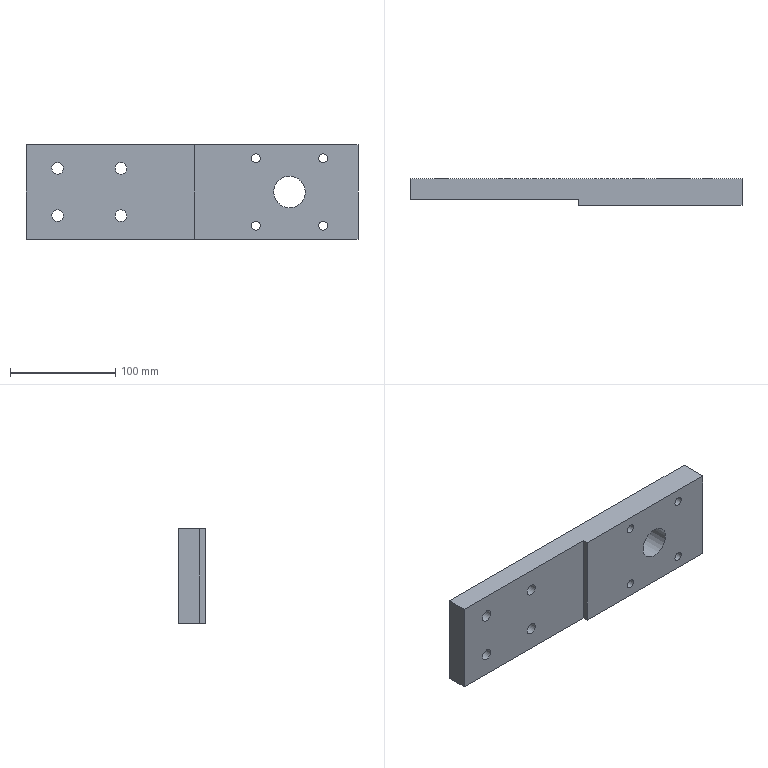Part | STEP file | SN10_002_001_PLACA | 1 solid | 17 faces | box 315 x 25 x 90 mm | volume 605966 mm3 | cylinder 9 | plane 8 | commonest cylinder face diameters 8.376 x4 11 x4 30 x1
STEP:
#1=CARTESIAN_POINT('',(0.,0.,0.));
#2=DIRECTION('',(0.,0.,1.));
#3=DIRECTION('',(1.,0.,0.));
#4=AXIS2_PLACEMENT_3D('',#1,#2,#3);
#5=CARTESIAN_POINT('',(5784.827,200.,-19.863));
#6=VERTEX_POINT('',#5);
#7=CARTESIAN_POINT('',(5780.,200.,-22.5));
#8=DIRECTION('',(0.,-1.,0.));
#9=DIRECTION('',(1.,0.,0.));
#10=AXIS2_PLACEMENT_3D('',#7,#8,#9);
#11=CIRCLE('',#10,5.5);
#12=CARTESIAN_POINT('',(5780.,199.9,-22.5));
#13=DIRECTION('',(0.,-1.,0.));
#14=DIRECTION('',(0.8776,0.,0.4794));
#15=AXIS2_PLACEMENT_3D('',#12,#13,#14);
#16=CYLINDRICAL_SURFACE('',#15,5.5);
#17=CARTESIAN_POINT('',(-0.5,-0.1));
#18=DIRECTION('',(1.,0.));
#19=VECTOR('',#18,1.);
#20=LINE('',#17,#19);
#21=(GEOMETRIC_REPRESENTATION_CONTEXT(2)PARAMETRIC_REPRESENTATION_CONTEXT()REPRESENTATION_CONTEXT('',''));
#22=DEFINITIONAL_REPRESENTATION('',(#20),#21);
#23=PCURVE('',#16,#22);
#24=CARTESIAN_POINT('',(6065.,200.,0.));
#25=DIRECTION('',(0.,1.,0.));
#26=DIRECTION('',(0.,0.,1.));
#27=AXIS2_PLACEMENT_3D('',#24,#25,#26);
#28=PLANE('',#27);
#29=CARTESIAN_POINT('',(-22.5,-279.5));
#30=CARTESIAN_POINT('',(-12.974,-279.5));
#31=CARTESIAN_POINT('',(-17.737,-287.75));
#32=CARTESIAN_POINT('',(-22.5,-296.));
#33=CARTESIAN_POINT('',(-27.263,-287.75));
#34=CARTESIAN_POINT('',(-32.026,-279.5));
#35=CARTESIAN_POINT('',(-22.5,-279.5));
#36=(BOUNDED_CURVE()B_SPLINE_CURVE(2,(#29,#30,#31,#32,#33,#34,#35),.UNSPECIFIED.,.T.,.F.)B_SPLINE_CURVE_WITH_KNOTS((1,2,2,2,2,1),(-2.094,0.,2.094,4.189,6.283,8.378),.UNSPECIFIED.)CURVE()GEOMETRIC_REPRESENTATION_ITEM()RATIONAL_B_SPLINE_CURVE((1.,0.5,1.,0.5,1.,0.5,1.))REPRESENTATION_ITEM(''));
#37=(GEOMETRIC_REPRESENTATION_CONTEXT(2)PARAMETRIC_REPRESENTATION_CONTEXT()REPRESENTATION_CONTEXT('',''));
#38=DEFINITIONAL_REPRESENTATION('',(#36),#37);
#39=PCURVE('',#28,#38);
#40=SURFACE_CURVE('',#11,(#23,#39),.PCURVE_S1.);
#41=EDGE_CURVE('',#6,#6,#40,.T.);
#42=ORIENTED_EDGE('',*,*,#41,.T.);
#43=CARTESIAN_POINT('',(5784.827,180.,-19.863));
#44=VERTEX_POINT('',#43);
#45=CARTESIAN_POINT('',(5784.827,200.,-19.863));
#46=CARTESIAN_POINT('',(5784.827,180.,-19.863));
#47=B_SPLINE_CURVE_WITH_KNOTS('',1,(#45,#46),.UNSPECIFIED.,.F.,.F.,(2,2),(-0.1,19.9),.PIECEWISE_BEZIER_KNOTS.);
#48=CARTESIAN_POINT('',(6.283,0.));
#49=DIRECTION('',(0.,1.));
#50=VECTOR('',#49,1.);
#51=LINE('',#48,#50);
#52=(GEOMETRIC_REPRESENTATION_CONTEXT(2)PARAMETRIC_REPRESENTATION_CONTEXT()REPRESENTATION_CONTEXT('',''));
#53=DEFINITIONAL_REPRESENTATION('',(#51),#52);
#54=PCURVE('',#16,#53);
#55=CARTESIAN_POINT('',(0.,0.));
#56=DIRECTION('',(0.,1.));
#57=VECTOR('',#56,1.);
#58=LINE('',#55,#57);
#59=(GEOMETRIC_REPRESENTATION_CONTEXT(2)PARAMETRIC_REPRESENTATION_CONTEXT()REPRESENTATION_CONTEXT('',''));
#60=DEFINITIONAL_REPRESENTATION('',(#58),#59);
#61=PCURVE('',#16,#60);
#62=SEAM_CURVE('',#47,(#54,#61),.PCURVE_S1.);
#63=EDGE_CURVE('',#6,#44,#62,.T.);
#64=ORIENTED_EDGE('',*,*,#63,.T.);
#65=CARTESIAN_POINT('',(5780.,180.,-22.5));
#66=DIRECTION('',(0.,-1.,0.));
#67=DIRECTION('',(1.,0.,0.));
#68=AXIS2_PLACEMENT_3D('',#65,#66,#67);
#69=CIRCLE('',#68,5.5);
#70=CARTESIAN_POINT('',(-0.5,19.9));
#71=DIRECTION('',(1.,0.));
#72=VECTOR('',#71,1.);
#73=LINE('',#70,#72);
#74=(GEOMETRIC_REPRESENTATION_CONTEXT(2)PARAMETRIC_REPRESENTATION_CONTEXT()REPRESENTATION_CONTEXT('',''));
#75=DEFINITIONAL_REPRESENTATION('',(#73),#74);
#76=PCURVE('',#16,#75);
#77=CARTESIAN_POINT('',(5750.,180.,0.));
#78=DIRECTION('',(0.,-1.,0.));
#79=DIRECTION('',(0.,0.,-1.));
#80=AXIS2_PLACEMENT_3D('',#77,#78,#79);
#81=PLANE('',#80);
#82=CARTESIAN_POINT('',(22.5,30.));
#83=DIRECTION('',(0.,1.));
#84=AXIS2_PLACEMENT_2D('',#82,#83);
#85=CIRCLE('',#84,5.5);
#86=(GEOMETRIC_REPRESENTATION_CONTEXT(2)PARAMETRIC_REPRESENTATION_CONTEXT()REPRESENTATION_CONTEXT('',''));
#87=DEFINITIONAL_REPRESENTATION('',(#85),#86);
#88=PCURVE('',#81,#87);
#89=SURFACE_CURVE('',#69,(#76,#88),.PCURVE_S1.);
#90=EDGE_CURVE('',#44,#44,#89,.T.);
#91=ORIENTED_EDGE('',*,*,#90,.F.);
#92=ORIENTED_EDGE('',*,*,#63,.F.);
#93=EDGE_LOOP('',(#42,#64,#91,#92));
#94=FACE_BOUND('',#93,.F.);
#95=ADVANCED_FACE('',(#94),#16,.F.);
#96=CARTESIAN_POINT('',(5750.,200.,-45.));
#97=VERTEX_POINT('',#96);
#98=CARTESIAN_POINT('',(5750.,180.,-45.));
#99=VERTEX_POINT('',#98);
#100=CARTESIAN_POINT('',(5750.,200.,-45.));
#101=DIRECTION('',(0.,-1.,0.));
#102=VECTOR('',#101,1.);
#103=LINE('',#100,#102);
#104=CARTESIAN_POINT('',(0.,0.,-45.));
#105=DIRECTION('',(0.,0.,1.));
#106=DIRECTION('',(1.,0.,0.));
#107=AXIS2_PLACEMENT_3D('',#104,#105,#106);
#108=PLANE('',#107);
#109=CARTESIAN_POINT('',(5750.,200.));
#110=DIRECTION('',(0.,-1.));
#111=VECTOR('',#110,1.);
#112=LINE('',#109,#111);
#113=(GEOMETRIC_REPRESENTATION_CONTEXT(2)PARAMETRIC_REPRESENTATION_CONTEXT()REPRESENTATION_CONTEXT('',''));
#114=DEFINITIONAL_REPRESENTATION('',(#112),#113);
#115=PCURVE('',#108,#114);
#116=CARTESIAN_POINT('',(5750.,200.,0.));
#117=DIRECTION('',(-1.,0.,0.));
#118=DIRECTION('',(0.,0.,1.));
#119=AXIS2_PLACEMENT_3D('',#116,#117,#118);
#120=PLANE('',#119);
#121=CARTESIAN_POINT('',(-45.,0.));
#122=DIRECTION('',(0.,-1.));
#123=VECTOR('',#122,1.);
#124=LINE('',#121,#123);
#125=(GEOMETRIC_REPRESENTATION_CONTEXT(2)PARAMETRIC_REPRESENTATION_CONTEXT()REPRESENTATION_CONTEXT('',''));
#126=DEFINITIONAL_REPRESENTATION('',(#124),#125);
#127=PCURVE('',#120,#126);
#128=SURFACE_CURVE('',#103,(#115,#127),.PCURVE_S1.);
#129=EDGE_CURVE('',#97,#99,#128,.T.);
#130=ORIENTED_EDGE('',*,*,#129,.F.);
#131=CARTESIAN_POINT('',(6065.,200.,-45.));
#132=VERTEX_POINT('',#131);
#133=CARTESIAN_POINT('',(6065.,200.,-45.));
#134=DIRECTION('',(-1.,0.,0.));
#135=VECTOR('',#134,1.);
#136=LINE('',#133,#135);
#137=CARTESIAN_POINT('',(6065.,200.));
#138=DIRECTION('',(-1.,0.));
#139=VECTOR('',#138,1.);
#140=LINE('',#137,#139);
#141=(GEOMETRIC_REPRESENTATION_CONTEXT(2)PARAMETRIC_REPRESENTATION_CONTEXT()REPRESENTATION_CONTEXT('',''));
#142=DEFINITIONAL_REPRESENTATION('',(#140),#141);
#143=PCURVE('',#108,#142);
#144=CARTESIAN_POINT('',(-45.,0.));
#145=DIRECTION('',(0.,-1.));
#146=VECTOR('',#145,1.);
#147=LINE('',#144,#146);
#148=(GEOMETRIC_REPRESENTATION_CONTEXT(2)PARAMETRIC_REPRESENTATION_CONTEXT()REPRESENTATION_CONTEXT('',''));
#149=DEFINITIONAL_REPRESENTATION('',(#147),#148);
#150=PCURVE('',#28,#149);
#151=SURFACE_CURVE('',#136,(#143,#150),.PCURVE_S1.);
#152=EDGE_CURVE('',#132,#97,#151,.T.);
#153=ORIENTED_EDGE('',*,*,#152,.F.);
#154=CARTESIAN_POINT('',(6065.,175.,-45.));
#155=VERTEX_POINT('',#154);
#156=CARTESIAN_POINT('',(6065.,175.,-45.));
#157=DIRECTION('',(0.,1.,0.));
#158=VECTOR('',#157,1.);
#159=LINE('',#156,#158);
#160=CARTESIAN_POINT('',(6065.,175.));
#161=DIRECTION('',(0.,1.));
#162=VECTOR('',#161,1.);
#163=LINE('',#160,#162);
#164=(GEOMETRIC_REPRESENTATION_CONTEXT(2)PARAMETRIC_REPRESENTATION_CONTEXT()REPRESENTATION_CONTEXT('',''));
#165=DEFINITIONAL_REPRESENTATION('',(#163),#164);
#166=PCURVE('',#108,#165);
#167=CARTESIAN_POINT('',(6065.,175.,0.));
#168=DIRECTION('',(1.,0.,0.));
#169=DIRECTION('',(0.,0.,-1.));
#170=AXIS2_PLACEMENT_3D('',#167,#168,#169);
#171=PLANE('',#170);
#172=CARTESIAN_POINT('',(45.,0.));
#173=DIRECTION('',(0.,1.));
#174=VECTOR('',#173,1.);
#175=LINE('',#172,#174);
#176=(GEOMETRIC_REPRESENTATION_CONTEXT(2)PARAMETRIC_REPRESENTATION_CONTEXT()REPRESENTATION_CONTEXT('',''));
#177=DEFINITIONAL_REPRESENTATION('',(#175),#176);
#178=PCURVE('',#171,#177);
#179=SURFACE_CURVE('',#159,(#166,#178),.PCURVE_S1.);
#180=EDGE_CURVE('',#155,#132,#179,.T.);
#181=ORIENTED_EDGE('',*,*,#180,.F.);
#182=CARTESIAN_POINT('',(5910.,175.,-45.));
#183=VERTEX_POINT('',#182);
#184=CARTESIAN_POINT('',(5910.,175.,-45.));
#185=DIRECTION('',(1.,0.,0.));
#186=VECTOR('',#185,1.);
#187=LINE('',#184,#186);
#188=CARTESIAN_POINT('',(5910.,175.));
#189=DIRECTION('',(1.,0.));
#190=VECTOR('',#189,1.);
#191=LINE('',#188,#190);
#192=(GEOMETRIC_REPRESENTATION_CONTEXT(2)PARAMETRIC_REPRESENTATION_CONTEXT()REPRESENTATION_CONTEXT('',''));
#193=DEFINITIONAL_REPRESENTATION('',(#191),#192);
#194=PCURVE('',#108,#193);
#195=CARTESIAN_POINT('',(5910.,175.,0.));
#196=DIRECTION('',(0.,-1.,0.));
#197=DIRECTION('',(0.,0.,-1.));
#198=AXIS2_PLACEMENT_3D('',#195,#196,#197);
#199=PLANE('',#198);
#200=CARTESIAN_POINT('',(45.,0.));
#201=DIRECTION('',(0.,1.));
#202=VECTOR('',#201,1.);
#203=LINE('',#200,#202);
#204=(GEOMETRIC_REPRESENTATION_CONTEXT(2)PARAMETRIC_REPRESENTATION_CONTEXT()REPRESENTATION_CONTEXT('',''));
#205=DEFINITIONAL_REPRESENTATION('',(#203),#204);
#206=PCURVE('',#199,#205);
#207=SURFACE_CURVE('',#187,(#194,#206),.PCURVE_S1.);
#208=EDGE_CURVE('',#183,#155,#207,.T.);
#209=ORIENTED_EDGE('',*,*,#208,.F.);
#210=CARTESIAN_POINT('',(5910.,180.,-45.));
#211=VERTEX_POINT('',#210);
#212=CARTESIAN_POINT('',(5910.,180.,-45.));
#213=DIRECTION('',(0.,-1.,0.));
#214=VECTOR('',#213,1.);
#215=LINE('',#212,#214);
#216=CARTESIAN_POINT('',(5910.,180.));
#217=DIRECTION('',(0.,-1.));
#218=VECTOR('',#217,1.);
#219=LINE('',#216,#218);
#220=(GEOMETRIC_REPRESENTATION_CONTEXT(2)PARAMETRIC_REPRESENTATION_CONTEXT()REPRESENTATION_CONTEXT('',''));
#221=DEFINITIONAL_REPRESENTATION('',(#219),#220);
#222=PCURVE('',#108,#221);
#223=CARTESIAN_POINT('',(5910.,180.,0.));
#224=DIRECTION('',(-1.,0.,0.));
#225=DIRECTION('',(0.,0.,1.));
#226=AXIS2_PLACEMENT_3D('',#223,#224,#225);
#227=PLANE('',#226);
#228=CARTESIAN_POINT('',(-45.,0.));
#229=DIRECTION('',(0.,-1.));
#230=VECTOR('',#229,1.);
#231=LINE('',#228,#230);
#232=(GEOMETRIC_REPRESENTATION_CONTEXT(2)PARAMETRIC_REPRESENTATION_CONTEXT()REPRESENTATION_CONTEXT('',''));
#233=DEFINITIONAL_REPRESENTATION('',(#231),#232);
#234=PCURVE('',#227,#233);
#235=SURFACE_CURVE('',#215,(#222,#234),.PCURVE_S1.);
#236=EDGE_CURVE('',#211,#183,#235,.T.);
#237=ORIENTED_EDGE('',*,*,#236,.F.);
#238=CARTESIAN_POINT('',(5750.,180.,-45.));
#239=DIRECTION('',(1.,0.,0.));
#240=VECTOR('',#239,1.);
#241=LINE('',#238,#240);
#242=CARTESIAN_POINT('',(5750.,180.));
#243=DIRECTION('',(1.,0.));
#244=VECTOR('',#243,1.);
#245=LINE('',#242,#244);
#246=(GEOMETRIC_REPRESENTATION_CONTEXT(2)PARAMETRIC_REPRESENTATION_CONTEXT()REPRESENTATION_CONTEXT('',''));
#247=DEFINITIONAL_REPRESENTATION('',(#245),#246);
#248=PCURVE('',#108,#247);
#249=CARTESIAN_POINT('',(45.,0.));
#250=DIRECTION('',(0.,1.));
#251=VECTOR('',#250,1.);
#252=LINE('',#249,#251);
#253=(GEOMETRIC_REPRESENTATION_CONTEXT(2)PARAMETRIC_REPRESENTATION_CONTEXT()REPRESENTATION_CONTEXT('',''));
#254=DEFINITIONAL_REPRESENTATION('',(#252),#253);
#255=PCURVE('',#81,#254);
#256=SURFACE_CURVE('',#241,(#248,#255),.PCURVE_S1.);
#257=EDGE_CURVE('',#99,#211,#256,.T.);
#258=ORIENTED_EDGE('',*,*,#257,.F.);
#259=EDGE_LOOP('',(#130,#153,#181,#209,#237,#258));
#260=FACE_BOUND('',#259,.T.);
#261=ADVANCED_FACE('',(#260),#108,.F.);
#262=CARTESIAN_POINT('',(5750.,200.,45.));
#263=VERTEX_POINT('',#262);
#264=CARTESIAN_POINT('',(5750.,200.,-45.));
#265=DIRECTION('',(0.,0.,1.));
#266=VECTOR('',#265,1.);
#267=LINE('',#264,#266);
#268=CARTESIAN_POINT('',(-45.,0.));
#269=DIRECTION('',(1.,0.));
#270=VECTOR('',#269,1.);
#271=LINE('',#268,#270);
#272=(GEOMETRIC_REPRESENTATION_CONTEXT(2)PARAMETRIC_REPRESENTATION_CONTEXT()REPRESENTATION_CONTEXT('',''));
#273=DEFINITIONAL_REPRESENTATION('',(#271),#272);
#274=PCURVE('',#120,#273);
#275=CARTESIAN_POINT('',(-45.,-315.));
#276=DIRECTION('',(1.,0.));
#277=VECTOR('',#276,1.);
#278=LINE('',#275,#277);
#279=(GEOMETRIC_REPRESENTATION_CONTEXT(2)PARAMETRIC_REPRESENTATION_CONTEXT()REPRESENTATION_CONTEXT('',''));
#280=DEFINITIONAL_REPRESENTATION('',(#278),#279);
#281=PCURVE('',#28,#280);
#282=SURFACE_CURVE('',#267,(#274,#281),.PCURVE_S1.);
#283=EDGE_CURVE('',#97,#263,#282,.T.);
#284=ORIENTED_EDGE('',*,*,#283,.F.);
#285=ORIENTED_EDGE('',*,*,#129,.T.);
#286=CARTESIAN_POINT('',(5750.,180.,45.));
#287=VERTEX_POINT('',#286);
#288=CARTESIAN_POINT('',(5750.,180.,-45.));
#289=DIRECTION('',(0.,0.,1.));
#290=VECTOR('',#289,1.);
#291=LINE('',#288,#290);
#292=CARTESIAN_POINT('',(-45.,-20.));
#293=DIRECTION('',(1.,0.));
#294=VECTOR('',#293,1.);
#295=LINE('',#292,#294);
#296=(GEOMETRIC_REPRESENTATION_CONTEXT(2)PARAMETRIC_REPRESENTATION_CONTEXT()REPRESENTATION_CONTEXT('',''));
#297=DEFINITIONAL_REPRESENTATION('',(#295),#296);
#298=PCURVE('',#120,#297);
#299=CARTESIAN_POINT('',(45.,0.));
#300=DIRECTION('',(-1.,0.));
#301=VECTOR('',#300,1.);
#302=LINE('',#299,#301);
#303=(GEOMETRIC_REPRESENTATION_CONTEXT(2)PARAMETRIC_REPRESENTATION_CONTEXT()REPRESENTATION_CONTEXT('',''));
#304=DEFINITIONAL_REPRESENTATION('',(#302),#303);
#305=PCURVE('',#81,#304);
#306=SURFACE_CURVE('',#291,(#298,#305),.PCURVE_S1.);
#307=EDGE_CURVE('',#99,#287,#306,.T.);
#308=ORIENTED_EDGE('',*,*,#307,.T.);
#309=CARTESIAN_POINT('',(5750.,200.,45.));
#310=DIRECTION('',(0.,-1.,0.));
#311=VECTOR('',#310,1.);
#312=LINE('',#309,#311);
#313=CARTESIAN_POINT('',(45.,0.));
#314=DIRECTION('',(0.,-1.));
#315=VECTOR('',#314,1.);
#316=LINE('',#313,#315);
#317=(GEOMETRIC_REPRESENTATION_CONTEXT(2)PARAMETRIC_REPRESENTATION_CONTEXT()REPRESENTATION_CONTEXT('',''));
#318=DEFINITIONAL_REPRESENTATION('',(#316),#317);
#319=PCURVE('',#120,#318);
#320=CARTESIAN_POINT('',(0.,0.,45.));
#321=DIRECTION('',(0.,0.,1.));
#322=DIRECTION('',(1.,0.,0.));
#323=AXIS2_PLACEMENT_3D('',#320,#321,#322);
#324=PLANE('',#323);
#325=CARTESIAN_POINT('',(5750.,200.));
#326=DIRECTION('',(0.,-1.));
#327=VECTOR('',#326,1.);
#328=LINE('',#325,#327);
#329=(GEOMETRIC_REPRESENTATION_CONTEXT(2)PARAMETRIC_REPRESENTATION_CONTEXT()REPRESENTATION_CONTEXT('',''));
#330=DEFINITIONAL_REPRESENTATION('',(#328),#329);
#331=PCURVE('',#324,#330);
#332=SURFACE_CURVE('',#312,(#319,#331),.PCURVE_S1.);
#333=EDGE_CURVE('',#263,#287,#332,.T.);
#334=ORIENTED_EDGE('',*,*,#333,.F.);
#335=EDGE_LOOP('',(#284,#285,#308,#334));
#336=FACE_BOUND('',#335,.T.);
#337=ADVANCED_FACE('',(#336),#120,.T.);
#338=CARTESIAN_POINT('',(5910.,180.,45.));
#339=VERTEX_POINT('',#338);
#340=CARTESIAN_POINT('',(5910.,180.,-45.));
#341=DIRECTION('',(0.,0.,1.));
#342=VECTOR('',#341,1.);
#343=LINE('',#340,#342);
#344=CARTESIAN_POINT('',(-45.,0.));
#345=DIRECTION('',(1.,0.));
#346=VECTOR('',#345,1.);
#347=LINE('',#344,#346);
#348=(GEOMETRIC_REPRESENTATION_CONTEXT(2)PARAMETRIC_REPRESENTATION_CONTEXT()REPRESENTATION_CONTEXT('',''));
#349=DEFINITIONAL_REPRESENTATION('',(#347),#348);
#350=PCURVE('',#227,#349);
#351=CARTESIAN_POINT('',(45.,160.));
#352=DIRECTION('',(-1.,0.));
#353=VECTOR('',#352,1.);
#354=LINE('',#351,#353);
#355=(GEOMETRIC_REPRESENTATION_CONTEXT(2)PARAMETRIC_REPRESENTATION_CONTEXT()REPRESENTATION_CONTEXT('',''));
#356=DEFINITIONAL_REPRESENTATION('',(#354),#355);
#357=PCURVE('',#81,#356);
#358=SURFACE_CURVE('',#343,(#350,#357),.PCURVE_S1.);
#359=EDGE_CURVE('',#211,#339,#358,.T.);
#360=ORIENTED_EDGE('',*,*,#359,.F.);
#361=ORIENTED_EDGE('',*,*,#236,.T.);
#362=CARTESIAN_POINT('',(5910.,175.,45.));
#363=VERTEX_POINT('',#362);
#364=CARTESIAN_POINT('',(5910.,175.,-45.));
#365=DIRECTION('',(0.,0.,1.));
#366=VECTOR('',#365,1.);
#367=LINE('',#364,#366);
#368=CARTESIAN_POINT('',(-45.,-5.));
#369=DIRECTION('',(1.,0.));
#370=VECTOR('',#369,1.);
#371=LINE('',#368,#370);
#372=(GEOMETRIC_REPRESENTATION_CONTEXT(2)PARAMETRIC_REPRESENTATION_CONTEXT()REPRESENTATION_CONTEXT('',''));
#373=DEFINITIONAL_REPRESENTATION('',(#371),#372);
#374=PCURVE('',#227,#373);
#375=CARTESIAN_POINT('',(45.,0.));
#376=DIRECTION('',(-1.,0.));
#377=VECTOR('',#376,1.);
#378=LINE('',#375,#377);
#379=(GEOMETRIC_REPRESENTATION_CONTEXT(2)PARAMETRIC_REPRESENTATION_CONTEXT()REPRESENTATION_CONTEXT('',''));
#380=DEFINITIONAL_REPRESENTATION('',(#378),#379);
#381=PCURVE('',#199,#380);
#382=SURFACE_CURVE('',#367,(#374,#381),.PCURVE_S1.);
#383=EDGE_CURVE('',#183,#363,#382,.T.);
#384=ORIENTED_EDGE('',*,*,#383,.T.);
#385=CARTESIAN_POINT('',(5910.,180.,45.));
#386=DIRECTION('',(0.,-1.,0.));
#387=VECTOR('',#386,1.);
#388=LINE('',#385,#387);
#389=CARTESIAN_POINT('',(45.,0.));
#390=DIRECTION('',(0.,-1.));
#391=VECTOR('',#390,1.);
#392=LINE('',#389,#391);
#393=(GEOMETRIC_REPRESENTATION_CONTEXT(2)PARAMETRIC_REPRESENTATION_CONTEXT()REPRESENTATION_CONTEXT('',''));
#394=DEFINITIONAL_REPRESENTATION('',(#392),#393);
#395=PCURVE('',#227,#394);
#396=CARTESIAN_POINT('',(5910.,180.));
#397=DIRECTION('',(0.,-1.));
#398=VECTOR('',#397,1.);
#399=LINE('',#396,#398);
#400=(GEOMETRIC_REPRESENTATION_CONTEXT(2)PARAMETRIC_REPRESENTATION_CONTEXT()REPRESENTATION_CONTEXT('',''));
#401=DEFINITIONAL_REPRESENTATION('',(#399),#400);
#402=PCURVE('',#324,#401);
#403=SURFACE_CURVE('',#388,(#395,#402),.PCURVE_S1.);
#404=EDGE_CURVE('',#339,#363,#403,.T.);
#405=ORIENTED_EDGE('',*,*,#404,.F.);
#406=EDGE_LOOP('',(#360,#361,#384,#405));
#407=FACE_BOUND('',#406,.T.);
#408=ADVANCED_FACE('',(#407),#227,.T.);
#409=ORIENTED_EDGE('',*,*,#383,.F.);
#410=ORIENTED_EDGE('',*,*,#208,.T.);
#411=CARTESIAN_POINT('',(6065.,175.,45.));
#412=VERTEX_POINT('',#411);
#413=CARTESIAN_POINT('',(6065.,175.,-45.));
#414=DIRECTION('',(0.,0.,1.));
#415=VECTOR('',#414,1.);
#416=LINE('',#413,#415);
#417=CARTESIAN_POINT('',(45.,155.));
#418=DIRECTION('',(-1.,0.));
#419=VECTOR('',#418,1.);
#420=LINE('',#417,#419);
#421=(GEOMETRIC_REPRESENTATION_CONTEXT(2)PARAMETRIC_REPRESENTATION_CONTEXT()REPRESENTATION_CONTEXT('',''));
#422=DEFINITIONAL_REPRESENTATION('',(#420),#421);
#423=PCURVE('',#199,#422);
#424=CARTESIAN_POINT('',(45.,0.));
#425=DIRECTION('',(-1.,0.));
#426=VECTOR('',#425,1.);
#427=LINE('',#424,#426);
#428=(GEOMETRIC_REPRESENTATION_CONTEXT(2)PARAMETRIC_REPRESENTATION_CONTEXT()REPRESENTATION_CONTEXT('',''));
#429=DEFINITIONAL_REPRESENTATION('',(#427),#428);
#430=PCURVE('',#171,#429);
#431=SURFACE_CURVE('',#416,(#423,#430),.PCURVE_S1.);
#432=EDGE_CURVE('',#155,#412,#431,.T.);
#433=ORIENTED_EDGE('',*,*,#432,.T.);
#434=CARTESIAN_POINT('',(5910.,175.,45.));
#435=DIRECTION('',(1.,0.,0.));
#436=VECTOR('',#435,1.);
#437=LINE('',#434,#436);
#438=CARTESIAN_POINT('',(-45.,0.));
#439=DIRECTION('',(0.,1.));
#440=VECTOR('',#439,1.);
#441=LINE('',#438,#440);
#442=(GEOMETRIC_REPRESENTATION_CONTEXT(2)PARAMETRIC_REPRESENTATION_CONTEXT()REPRESENTATION_CONTEXT('',''));
#443=DEFINITIONAL_REPRESENTATION('',(#441),#442);
#444=PCURVE('',#199,#443);
#445=CARTESIAN_POINT('',(5910.,175.));
#446=DIRECTION('',(1.,0.));
#447=VECTOR('',#446,1.);
#448=LINE('',#445,#447);
#449=(GEOMETRIC_REPRESENTATION_CONTEXT(2)PARAMETRIC_REPRESENTATION_CONTEXT()REPRESENTATION_CONTEXT('',''));
#450=DEFINITIONAL_REPRESENTATION('',(#448),#449);
#451=PCURVE('',#324,#450);
#452=SURFACE_CURVE('',#437,(#444,#451),.PCURVE_S1.);
#453=EDGE_CURVE('',#363,#412,#452,.T.);
#454=ORIENTED_EDGE('',*,*,#453,.F.);
#455=EDGE_LOOP('',(#409,#410,#433,#454));
#456=FACE_BOUND('',#455,.T.);
#457=CARTESIAN_POINT('',(6035.675,175.,34.008));
#458=VERTEX_POINT('',#457);
#459=CARTESIAN_POINT('',(6032.,175.,32.));
#460=DIRECTION('',(0.,-1.,0.));
#461=DIRECTION('',(1.,0.,0.));
#462=AXIS2_PLACEMENT_3D('',#459,#460,#461);
#463=CIRCLE('',#462,4.188);
#464=CARTESIAN_POINT('',(-32.,122.));
#465=DIRECTION('',(0.,1.));
#466=AXIS2_PLACEMENT_2D('',#464,#465);
#467=CIRCLE('',#466,4.188);
#468=(GEOMETRIC_REPRESENTATION_CONTEXT(2)PARAMETRIC_REPRESENTATION_CONTEXT()REPRESENTATION_CONTEXT('',''));
#469=DEFINITIONAL_REPRESENTATION('',(#467),#468);
#470=PCURVE('',#199,#469);
#471=CARTESIAN_POINT('',(6032.,199.9,32.));
#472=DIRECTION('',(0.,-1.,0.));
#473=DIRECTION('',(0.8776,0.,0.4794));
#474=AXIS2_PLACEMENT_3D('',#471,#472,#473);
#475=CYLINDRICAL_SURFACE('',#474,4.188);
#476=CARTESIAN_POINT('',(-0.5,24.9));
#477=DIRECTION('',(1.,0.));
#478=VECTOR('',#477,1.);
#479=LINE('',#476,#478);
#480=(GEOMETRIC_REPRESENTATION_CONTEXT(2)PARAMETRIC_REPRESENTATION_CONTEXT()REPRESENTATION_CONTEXT('',''));
#481=DEFINITIONAL_REPRESENTATION('',(#479),#480);
#482=PCURVE('',#475,#481);
#483=SURFACE_CURVE('',#463,(#470,#482),.PCURVE_S1.);
#484=EDGE_CURVE('',#458,#458,#483,.T.);
#485=ORIENTED_EDGE('',*,*,#484,.F.);
#486=EDGE_LOOP('',(#485));
#487=FACE_BOUND('',#486,.T.);
#488=CARTESIAN_POINT('',(5971.675,175.,34.008));
#489=VERTEX_POINT('',#488);
#490=CARTESIAN_POINT('',(5968.,175.,32.));
#491=DIRECTION('',(0.,-1.,0.));
#492=DIRECTION('',(1.,0.,0.));
#493=AXIS2_PLACEMENT_3D('',#490,#491,#492);
#494=CIRCLE('',#493,4.188);
#495=CARTESIAN_POINT('',(-32.,58.));
#496=DIRECTION('',(0.,1.));
#497=AXIS2_PLACEMENT_2D('',#495,#496);
#498=CIRCLE('',#497,4.188);
#499=(GEOMETRIC_REPRESENTATION_CONTEXT(2)PARAMETRIC_REPRESENTATION_CONTEXT()REPRESENTATION_CONTEXT('',''));
#500=DEFINITIONAL_REPRESENTATION('',(#498),#499);
#501=PCURVE('',#199,#500);
#502=CARTESIAN_POINT('',(5968.,199.9,32.));
#503=DIRECTION('',(0.,-1.,0.));
#504=DIRECTION('',(0.8776,0.,0.4794));
#505=AXIS2_PLACEMENT_3D('',#502,#503,#504);
#506=CYLINDRICAL_SURFACE('',#505,4.188);
#507=CARTESIAN_POINT('',(-0.5,24.9));
#508=DIRECTION('',(1.,0.));
#509=VECTOR('',#508,1.);
#510=LINE('',#507,#509);
#511=(GEOMETRIC_REPRESENTATION_CONTEXT(2)PARAMETRIC_REPRESENTATION_CONTEXT()REPRESENTATION_CONTEXT('',''));
#512=DEFINITIONAL_REPRESENTATION('',(#510),#511);
#513=PCURVE('',#506,#512);
#514=SURFACE_CURVE('',#494,(#501,#513),.PCURVE_S1.);
#515=EDGE_CURVE('',#489,#489,#514,.T.);
#516=ORIENTED_EDGE('',*,*,#515,.F.);
#517=EDGE_LOOP('',(#516));
#518=FACE_BOUND('',#517,.T.);
#519=CARTESIAN_POINT('',(5971.675,175.,-29.992));
#520=VERTEX_POINT('',#519);
#521=CARTESIAN_POINT('',(5968.,175.,-32.));
#522=DIRECTION('',(0.,-1.,0.));
#523=DIRECTION('',(1.,0.,0.));
#524=AXIS2_PLACEMENT_3D('',#521,#522,#523);
#525=CIRCLE('',#524,4.188);
#526=CARTESIAN_POINT('',(32.,58.));
#527=DIRECTION('',(0.,1.));
#528=AXIS2_PLACEMENT_2D('',#526,#527);
#529=CIRCLE('',#528,4.188);
#530=(GEOMETRIC_REPRESENTATION_CONTEXT(2)PARAMETRIC_REPRESENTATION_CONTEXT()REPRESENTATION_CONTEXT('',''));
#531=DEFINITIONAL_REPRESENTATION('',(#529),#530);
#532=PCURVE('',#199,#531);
#533=CARTESIAN_POINT('',(5968.,199.9,-32.));
#534=DIRECTION('',(0.,-1.,0.));
#535=DIRECTION('',(0.8776,0.,0.4794));
#536=AXIS2_PLACEMENT_3D('',#533,#534,#535);
#537=CYLINDRICAL_SURFACE('',#536,4.188);
#538=CARTESIAN_POINT('',(-0.5,24.9));
#539=DIRECTION('',(1.,0.));
#540=VECTOR('',#539,1.);
#541=LINE('',#538,#540);
#542=(GEOMETRIC_REPRESENTATION_CONTEXT(2)PARAMETRIC_REPRESENTATION_CONTEXT()REPRESENTATION_CONTEXT('',''));
#543=DEFINITIONAL_REPRESENTATION('',(#541),#542);
#544=PCURVE('',#537,#543);
#545=SURFACE_CURVE('',#525,(#532,#544),.PCURVE_S1.);
#546=EDGE_CURVE('',#520,#520,#545,.T.);
#547=ORIENTED_EDGE('',*,*,#546,.F.);
#548=EDGE_LOOP('',(#547));
#549=FACE_BOUND('',#548,.T.);
#550=CARTESIAN_POINT('',(6035.675,175.,-29.992));
#551=VERTEX_POINT('',#550);
#552=CARTESIAN_POINT('',(6032.,175.,-32.));
#553=DIRECTION('',(0.,-1.,0.));
#554=DIRECTION('',(1.,0.,0.));
#555=AXIS2_PLACEMENT_3D('',#552,#553,#554);
#556=CIRCLE('',#555,4.188);
#557=CARTESIAN_POINT('',(32.,122.));
#558=DIRECTION('',(0.,1.));
#559=AXIS2_PLACEMENT_2D('',#557,#558);
#560=CIRCLE('',#559,4.188);
#561=(GEOMETRIC_REPRESENTATION_CONTEXT(2)PARAMETRIC_REPRESENTATION_CONTEXT()REPRESENTATION_CONTEXT('',''));
#562=DEFINITIONAL_REPRESENTATION('',(#560),#561);
#563=PCURVE('',#199,#562);
#564=CARTESIAN_POINT('',(6032.,199.9,-32.));
#565=DIRECTION('',(0.,-1.,0.));
#566=DIRECTION('',(0.8776,0.,0.4794));
#567=AXIS2_PLACEMENT_3D('',#564,#565,#566);
#568=CYLINDRICAL_SURFACE('',#567,4.188);
#569=CARTESIAN_POINT('',(-0.5,24.9));
#570=DIRECTION('',(1.,0.));
#571=VECTOR('',#570,1.);
#572=LINE('',#569,#571);
#573=(GEOMETRIC_REPRESENTATION_CONTEXT(2)PARAMETRIC_REPRESENTATION_CONTEXT()REPRESENTATION_CONTEXT('',''));
#574=DEFINITIONAL_REPRESENTATION('',(#572),#573);
#575=PCURVE('',#568,#574);
#576=SURFACE_CURVE('',#556,(#563,#575),.PCURVE_S1.);
#577=EDGE_CURVE('',#551,#551,#576,.T.);
#578=ORIENTED_EDGE('',*,*,#577,.F.);
#579=EDGE_LOOP('',(#578));
#580=FACE_BOUND('',#579,.T.);
#581=CARTESIAN_POINT('',(6013.164,175.,7.191));
#582=VERTEX_POINT('',#581);
#583=CARTESIAN_POINT('',(6000.,175.,0.));
#584=DIRECTION('',(0.,-1.,0.));
#585=DIRECTION('',(1.,0.,0.));
#586=AXIS2_PLACEMENT_3D('',#583,#584,#585);
#587=CIRCLE('',#586,15.);
#588=CARTESIAN_POINT('',(0.,90.));
#589=DIRECTION('',(0.,1.));
#590=AXIS2_PLACEMENT_2D('',#588,#589);
#591=CIRCLE('',#590,15.);
#592=(GEOMETRIC_REPRESENTATION_CONTEXT(2)PARAMETRIC_REPRESENTATION_CONTEXT()REPRESENTATION_CONTEXT('',''));
#593=DEFINITIONAL_REPRESENTATION('',(#591),#592);
#594=PCURVE('',#199,#593);
#595=CARTESIAN_POINT('',(6000.,199.9,0.));
#596=DIRECTION('',(0.,-1.,0.));
#597=DIRECTION('',(0.8776,0.,0.4794));
#598=AXIS2_PLACEMENT_3D('',#595,#596,#597);
#599=CYLINDRICAL_SURFACE('',#598,15.);
#600=CARTESIAN_POINT('',(-0.5,24.9));
#601=DIRECTION('',(1.,0.));
#602=VECTOR('',#601,1.);
#603=LINE('',#600,#602);
#604=(GEOMETRIC_REPRESENTATION_CONTEXT(2)PARAMETRIC_REPRESENTATION_CONTEXT()REPRESENTATION_CONTEXT('',''));
#605=DEFINITIONAL_REPRESENTATION('',(#603),#604);
#606=PCURVE('',#599,#605);
#607=SURFACE_CURVE('',#587,(#594,#606),.PCURVE_S1.);
#608=EDGE_CURVE('',#582,#582,#607,.T.);
#609=ORIENTED_EDGE('',*,*,#608,.F.);
#610=EDGE_LOOP('',(#609));
#611=FACE_BOUND('',#610,.T.);
#612=ADVANCED_FACE('',(#456,#487,#518,#549,#580,#611),#199,.T.);
#613=CARTESIAN_POINT('',(6013.164,200.,7.191));
#614=VERTEX_POINT('',#613);
#615=CARTESIAN_POINT('',(6000.,200.,0.));
#616=DIRECTION('',(0.,-1.,0.));
#617=DIRECTION('',(1.,0.,0.));
#618=AXIS2_PLACEMENT_3D('',#615,#616,#617);
#619=CIRCLE('',#618,15.);
#620=CARTESIAN_POINT('',(-0.5,-0.1));
#621=DIRECTION('',(1.,0.));
#622=VECTOR('',#621,1.);
#623=LINE('',#620,#622);
#624=(GEOMETRIC_REPRESENTATION_CONTEXT(2)PARAMETRIC_REPRESENTATION_CONTEXT()REPRESENTATION_CONTEXT('',''));
#625=DEFINITIONAL_REPRESENTATION('',(#623),#624);
#626=PCURVE('',#599,#625);
#627=CARTESIAN_POINT('',(0.,-50.));
#628=CARTESIAN_POINT('',(25.981,-50.));
#629=CARTESIAN_POINT('',(12.99,-72.5));
#630=CARTESIAN_POINT('',(0.,-95.));
#631=CARTESIAN_POINT('',(-12.99,-72.5));
#632=CARTESIAN_POINT('',(-25.981,-50.));
#633=CARTESIAN_POINT('',(0.,-50.));
#634=(BOUNDED_CURVE()B_SPLINE_CURVE(2,(#627,#628,#629,#630,#631,#632,#633),.UNSPECIFIED.,.T.,.F.)B_SPLINE_CURVE_WITH_KNOTS((1,2,2,2,2,1),(-2.094,0.,2.094,4.189,6.283,8.378),.UNSPECIFIED.)CURVE()GEOMETRIC_REPRESENTATION_ITEM()RATIONAL_B_SPLINE_CURVE((1.,0.5,1.,0.5,1.,0.5,1.))REPRESENTATION_ITEM(''));
#635=(GEOMETRIC_REPRESENTATION_CONTEXT(2)PARAMETRIC_REPRESENTATION_CONTEXT()REPRESENTATION_CONTEXT('',''));
#636=DEFINITIONAL_REPRESENTATION('',(#634),#635);
#637=PCURVE('',#28,#636);
#638=SURFACE_CURVE('',#619,(#626,#637),.PCURVE_S1.);
#639=EDGE_CURVE('',#614,#614,#638,.T.);
#640=ORIENTED_EDGE('',*,*,#639,.T.);
#641=CARTESIAN_POINT('',(6013.164,200.,7.191));
#642=CARTESIAN_POINT('',(6013.164,175.,7.191));
#643=B_SPLINE_CURVE_WITH_KNOTS('',1,(#641,#642),.UNSPECIFIED.,.F.,.F.,(2,2),(-0.1,24.9),.PIECEWISE_BEZIER_KNOTS.);
#644=CARTESIAN_POINT('',(6.283,0.));
#645=DIRECTION('',(0.,1.));
#646=VECTOR('',#645,1.);
#647=LINE('',#644,#646);
#648=(GEOMETRIC_REPRESENTATION_CONTEXT(2)PARAMETRIC_REPRESENTATION_CONTEXT()REPRESENTATION_CONTEXT('',''));
#649=DEFINITIONAL_REPRESENTATION('',(#647),#648);
#650=PCURVE('',#599,#649);
#651=CARTESIAN_POINT('',(0.,0.));
#652=DIRECTION('',(0.,1.));
#653=VECTOR('',#652,1.);
#654=LINE('',#651,#653);
#655=(GEOMETRIC_REPRESENTATION_CONTEXT(2)PARAMETRIC_REPRESENTATION_CONTEXT()REPRESENTATION_CONTEXT('',''));
#656=DEFINITIONAL_REPRESENTATION('',(#654),#655);
#657=PCURVE('',#599,#656);
#658=SEAM_CURVE('',#643,(#650,#657),.PCURVE_S1.);
#659=EDGE_CURVE('',#614,#582,#658,.T.);
#660=ORIENTED_EDGE('',*,*,#659,.T.);
#661=ORIENTED_EDGE('',*,*,#608,.F.);
#662=ORIENTED_EDGE('',*,*,#659,.F.);
#663=EDGE_LOOP('',(#640,#660,#661,#662));
#664=FACE_BOUND('',#663,.F.);
#665=ADVANCED_FACE('',(#664),#599,.F.);
#666=CARTESIAN_POINT('',(6035.675,200.,-29.992));
#667=VERTEX_POINT('',#666);
#668=CARTESIAN_POINT('',(6032.,200.,-32.));
#669=DIRECTION('',(0.,-1.,0.));
#670=DIRECTION('',(1.,0.,0.));
#671=AXIS2_PLACEMENT_3D('',#668,#669,#670);
#672=CIRCLE('',#671,4.188);
#673=CARTESIAN_POINT('',(-0.5,-0.1));
#674=DIRECTION('',(1.,0.));
#675=VECTOR('',#674,1.);
#676=LINE('',#673,#675);
#677=(GEOMETRIC_REPRESENTATION_CONTEXT(2)PARAMETRIC_REPRESENTATION_CONTEXT()REPRESENTATION_CONTEXT('',''));
#678=DEFINITIONAL_REPRESENTATION('',(#676),#677);
#679=PCURVE('',#568,#678);
#680=CARTESIAN_POINT('',(-32.,-28.812));
#681=CARTESIAN_POINT('',(-24.746,-28.812));
#682=CARTESIAN_POINT('',(-28.373,-35.094));
#683=CARTESIAN_POINT('',(-32.,-41.376));
#684=CARTESIAN_POINT('',(-35.627,-35.094));
#685=CARTESIAN_POINT('',(-39.254,-28.812));
#686=CARTESIAN_POINT('',(-32.,-28.812));
#687=(BOUNDED_CURVE()B_SPLINE_CURVE(2,(#680,#681,#682,#683,#684,#685,#686),.UNSPECIFIED.,.T.,.F.)B_SPLINE_CURVE_WITH_KNOTS((1,2,2,2,2,1),(-2.094,0.,2.094,4.189,6.283,8.378),.UNSPECIFIED.)CURVE()GEOMETRIC_REPRESENTATION_ITEM()RATIONAL_B_SPLINE_CURVE((1.,0.5,1.,0.5,1.,0.5,1.))REPRESENTATION_ITEM(''));
#688=(GEOMETRIC_REPRESENTATION_CONTEXT(2)PARAMETRIC_REPRESENTATION_CONTEXT()REPRESENTATION_CONTEXT('',''));
#689=DEFINITIONAL_REPRESENTATION('',(#687),#688);
#690=PCURVE('',#28,#689);
#691=SURFACE_CURVE('',#672,(#679,#690),.PCURVE_S1.);
#692=EDGE_CURVE('',#667,#667,#691,.T.);
#693=ORIENTED_EDGE('',*,*,#692,.T.);
#694=CARTESIAN_POINT('',(6035.675,200.,-29.992));
#695=CARTESIAN_POINT('',(6035.675,175.,-29.992));
#696=B_SPLINE_CURVE_WITH_KNOTS('',1,(#694,#695),.UNSPECIFIED.,.F.,.F.,(2,2),(-0.1,24.9),.PIECEWISE_BEZIER_KNOTS.);
#697=CARTESIAN_POINT('',(6.283,0.));
#698=DIRECTION('',(0.,1.));
#699=VECTOR('',#698,1.);
#700=LINE('',#697,#699);
#701=(GEOMETRIC_REPRESENTATION_CONTEXT(2)PARAMETRIC_REPRESENTATION_CONTEXT()REPRESENTATION_CONTEXT('',''));
#702=DEFINITIONAL_REPRESENTATION('',(#700),#701);
#703=PCURVE('',#568,#702);
#704=CARTESIAN_POINT('',(0.,0.));
#705=DIRECTION('',(0.,1.));
#706=VECTOR('',#705,1.);
#707=LINE('',#704,#706);
#708=(GEOMETRIC_REPRESENTATION_CONTEXT(2)PARAMETRIC_REPRESENTATION_CONTEXT()REPRESENTATION_CONTEXT('',''));
#709=DEFINITIONAL_REPRESENTATION('',(#707),#708);
#710=PCURVE('',#568,#709);
#711=SEAM_CURVE('',#696,(#703,#710),.PCURVE_S1.);
#712=EDGE_CURVE('',#667,#551,#711,.T.);
#713=ORIENTED_EDGE('',*,*,#712,.T.);
#714=ORIENTED_EDGE('',*,*,#577,.F.);
#715=ORIENTED_EDGE('',*,*,#712,.F.);
#716=EDGE_LOOP('',(#693,#713,#714,#715));
#717=FACE_BOUND('',#716,.F.);
#718=ADVANCED_FACE('',(#717),#568,.F.);
#719=CARTESIAN_POINT('',(5971.675,200.,-29.992));
#720=VERTEX_POINT('',#719);
#721=CARTESIAN_POINT('',(5968.,200.,-32.));
#722=DIRECTION('',(0.,-1.,0.));
#723=DIRECTION('',(1.,0.,0.));
#724=AXIS2_PLACEMENT_3D('',#721,#722,#723);
#725=CIRCLE('',#724,4.188);
#726=CARTESIAN_POINT('',(-0.5,-0.1));
#727=DIRECTION('',(1.,0.));
#728=VECTOR('',#727,1.);
#729=LINE('',#726,#728);
#730=(GEOMETRIC_REPRESENTATION_CONTEXT(2)PARAMETRIC_REPRESENTATION_CONTEXT()REPRESENTATION_CONTEXT('',''));
#731=DEFINITIONAL_REPRESENTATION('',(#729),#730);
#732=PCURVE('',#537,#731);
#733=CARTESIAN_POINT('',(-32.,-92.812));
#734=CARTESIAN_POINT('',(-24.746,-92.812));
#735=CARTESIAN_POINT('',(-28.373,-99.094));
#736=CARTESIAN_POINT('',(-32.,-105.376));
#737=CARTESIAN_POINT('',(-35.627,-99.094));
#738=CARTESIAN_POINT('',(-39.254,-92.812));
#739=CARTESIAN_POINT('',(-32.,-92.812));
#740=(BOUNDED_CURVE()B_SPLINE_CURVE(2,(#733,#734,#735,#736,#737,#738,#739),.UNSPECIFIED.,.T.,.F.)B_SPLINE_CURVE_WITH_KNOTS((1,2,2,2,2,1),(-2.094,0.,2.094,4.189,6.283,8.378),.UNSPECIFIED.)CURVE()GEOMETRIC_REPRESENTATION_ITEM()RATIONAL_B_SPLINE_CURVE((1.,0.5,1.,0.5,1.,0.5,1.))REPRESENTATION_ITEM(''));
#741=(GEOMETRIC_REPRESENTATION_CONTEXT(2)PARAMETRIC_REPRESENTATION_CONTEXT()REPRESENTATION_CONTEXT('',''));
#742=DEFINITIONAL_REPRESENTATION('',(#740),#741);
#743=PCURVE('',#28,#742);
#744=SURFACE_CURVE('',#725,(#732,#743),.PCURVE_S1.);
#745=EDGE_CURVE('',#720,#720,#744,.T.);
#746=ORIENTED_EDGE('',*,*,#745,.T.);
#747=CARTESIAN_POINT('',(5971.675,200.,-29.992));
#748=CARTESIAN_POINT('',(5971.675,175.,-29.992));
#749=B_SPLINE_CURVE_WITH_KNOTS('',1,(#747,#748),.UNSPECIFIED.,.F.,.F.,(2,2),(-0.1,24.9),.PIECEWISE_BEZIER_KNOTS.);
#750=CARTESIAN_POINT('',(6.283,0.));
#751=DIRECTION('',(0.,1.));
#752=VECTOR('',#751,1.);
#753=LINE('',#750,#752);
#754=(GEOMETRIC_REPRESENTATION_CONTEXT(2)PARAMETRIC_REPRESENTATION_CONTEXT()REPRESENTATION_CONTEXT('',''));
#755=DEFINITIONAL_REPRESENTATION('',(#753),#754);
#756=PCURVE('',#537,#755);
#757=CARTESIAN_POINT('',(0.,0.));
#758=DIRECTION('',(0.,1.));
#759=VECTOR('',#758,1.);
#760=LINE('',#757,#759);
#761=(GEOMETRIC_REPRESENTATION_CONTEXT(2)PARAMETRIC_REPRESENTATION_CONTEXT()REPRESENTATION_CONTEXT('',''));
#762=DEFINITIONAL_REPRESENTATION('',(#760),#761);
#763=PCURVE('',#537,#762);
#764=SEAM_CURVE('',#749,(#756,#763),.PCURVE_S1.);
#765=EDGE_CURVE('',#720,#520,#764,.T.);
#766=ORIENTED_EDGE('',*,*,#765,.T.);
#767=ORIENTED_EDGE('',*,*,#546,.F.);
#768=ORIENTED_EDGE('',*,*,#765,.F.);
#769=EDGE_LOOP('',(#746,#766,#767,#768));
#770=FACE_BOUND('',#769,.F.);
#771=ADVANCED_FACE('',(#770),#537,.F.);
#772=CARTESIAN_POINT('',(5971.675,200.,34.008));
#773=VERTEX_POINT('',#772);
#774=CARTESIAN_POINT('',(5968.,200.,32.));
#775=DIRECTION('',(0.,-1.,0.));
#776=DIRECTION('',(1.,0.,0.));
#777=AXIS2_PLACEMENT_3D('',#774,#775,#776);
#778=CIRCLE('',#777,4.188);
#779=CARTESIAN_POINT('',(-0.5,-0.1));
#780=DIRECTION('',(1.,0.));
#781=VECTOR('',#780,1.);
#782=LINE('',#779,#781);
#783=(GEOMETRIC_REPRESENTATION_CONTEXT(2)PARAMETRIC_REPRESENTATION_CONTEXT()REPRESENTATION_CONTEXT('',''));
#784=DEFINITIONAL_REPRESENTATION('',(#782),#783);
#785=PCURVE('',#506,#784);
#786=CARTESIAN_POINT('',(32.,-92.812));
#787=CARTESIAN_POINT('',(39.254,-92.812));
#788=CARTESIAN_POINT('',(35.627,-99.094));
#789=CARTESIAN_POINT('',(32.,-105.376));
#790=CARTESIAN_POINT('',(28.373,-99.094));
#791=CARTESIAN_POINT('',(24.746,-92.812));
#792=CARTESIAN_POINT('',(32.,-92.812));
#793=(BOUNDED_CURVE()B_SPLINE_CURVE(2,(#786,#787,#788,#789,#790,#791,#792),.UNSPECIFIED.,.T.,.F.)B_SPLINE_CURVE_WITH_KNOTS((1,2,2,2,2,1),(-2.094,0.,2.094,4.189,6.283,8.378),.UNSPECIFIED.)CURVE()GEOMETRIC_REPRESENTATION_ITEM()RATIONAL_B_SPLINE_CURVE((1.,0.5,1.,0.5,1.,0.5,1.))REPRESENTATION_ITEM(''));
#794=(GEOMETRIC_REPRESENTATION_CONTEXT(2)PARAMETRIC_REPRESENTATION_CONTEXT()REPRESENTATION_CONTEXT('',''));
#795=DEFINITIONAL_REPRESENTATION('',(#793),#794);
#796=PCURVE('',#28,#795);
#797=SURFACE_CURVE('',#778,(#785,#796),.PCURVE_S1.);
#798=EDGE_CURVE('',#773,#773,#797,.T.);
#799=ORIENTED_EDGE('',*,*,#798,.T.);
#800=CARTESIAN_POINT('',(5971.675,200.,34.008));
#801=CARTESIAN_POINT('',(5971.675,175.,34.008));
#802=B_SPLINE_CURVE_WITH_KNOTS('',1,(#800,#801),.UNSPECIFIED.,.F.,.F.,(2,2),(-0.1,24.9),.PIECEWISE_BEZIER_KNOTS.);
#803=CARTESIAN_POINT('',(6.283,0.));
#804=DIRECTION('',(0.,1.));
#805=VECTOR('',#804,1.);
#806=LINE('',#803,#805);
#807=(GEOMETRIC_REPRESENTATION_CONTEXT(2)PARAMETRIC_REPRESENTATION_CONTEXT()REPRESENTATION_CONTEXT('',''));
#808=DEFINITIONAL_REPRESENTATION('',(#806),#807);
#809=PCURVE('',#506,#808);
#810=CARTESIAN_POINT('',(0.,0.));
#811=DIRECTION('',(0.,1.));
#812=VECTOR('',#811,1.);
#813=LINE('',#810,#812);
#814=(GEOMETRIC_REPRESENTATION_CONTEXT(2)PARAMETRIC_REPRESENTATION_CONTEXT()REPRESENTATION_CONTEXT('',''));
#815=DEFINITIONAL_REPRESENTATION('',(#813),#814);
#816=PCURVE('',#506,#815);
#817=SEAM_CURVE('',#802,(#809,#816),.PCURVE_S1.);
#818=EDGE_CURVE('',#773,#489,#817,.T.);
#819=ORIENTED_EDGE('',*,*,#818,.T.);
#820=ORIENTED_EDGE('',*,*,#515,.F.);
#821=ORIENTED_EDGE('',*,*,#818,.F.);
#822=EDGE_LOOP('',(#799,#819,#820,#821));
#823=FACE_BOUND('',#822,.F.);
#824=ADVANCED_FACE('',(#823),#506,.F.);
#825=CARTESIAN_POINT('',(6035.675,200.,34.008));
#826=VERTEX_POINT('',#825);
#827=CARTESIAN_POINT('',(6032.,200.,32.));
#828=DIRECTION('',(0.,-1.,0.));
#829=DIRECTION('',(1.,0.,0.));
#830=AXIS2_PLACEMENT_3D('',#827,#828,#829);
#831=CIRCLE('',#830,4.188);
#832=CARTESIAN_POINT('',(-0.5,-0.1));
#833=DIRECTION('',(1.,0.));
#834=VECTOR('',#833,1.);
#835=LINE('',#832,#834);
#836=(GEOMETRIC_REPRESENTATION_CONTEXT(2)PARAMETRIC_REPRESENTATION_CONTEXT()REPRESENTATION_CONTEXT('',''));
#837=DEFINITIONAL_REPRESENTATION('',(#835),#836);
#838=PCURVE('',#475,#837);
#839=CARTESIAN_POINT('',(32.,-28.812));
#840=CARTESIAN_POINT('',(39.254,-28.812));
#841=CARTESIAN_POINT('',(35.627,-35.094));
#842=CARTESIAN_POINT('',(32.,-41.376));
#843=CARTESIAN_POINT('',(28.373,-35.094));
#844=CARTESIAN_POINT('',(24.746,-28.812));
#845=CARTESIAN_POINT('',(32.,-28.812));
#846=(BOUNDED_CURVE()B_SPLINE_CURVE(2,(#839,#840,#841,#842,#843,#844,#845),.UNSPECIFIED.,.T.,.F.)B_SPLINE_CURVE_WITH_KNOTS((1,2,2,2,2,1),(-2.094,0.,2.094,4.189,6.283,8.378),.UNSPECIFIED.)CURVE()GEOMETRIC_REPRESENTATION_ITEM()RATIONAL_B_SPLINE_CURVE((1.,0.5,1.,0.5,1.,0.5,1.))REPRESENTATION_ITEM(''));
#847=(GEOMETRIC_REPRESENTATION_CONTEXT(2)PARAMETRIC_REPRESENTATION_CONTEXT()REPRESENTATION_CONTEXT('',''));
#848=DEFINITIONAL_REPRESENTATION('',(#846),#847);
#849=PCURVE('',#28,#848);
#850=SURFACE_CURVE('',#831,(#838,#849),.PCURVE_S1.);
#851=EDGE_CURVE('',#826,#826,#850,.T.);
#852=ORIENTED_EDGE('',*,*,#851,.T.);
#853=CARTESIAN_POINT('',(6035.675,200.,34.008));
#854=CARTESIAN_POINT('',(6035.675,175.,34.008));
#855=B_SPLINE_CURVE_WITH_KNOTS('',1,(#853,#854),.UNSPECIFIED.,.F.,.F.,(2,2),(-0.1,24.9),.PIECEWISE_BEZIER_KNOTS.);
#856=CARTESIAN_POINT('',(6.283,0.));
#857=DIRECTION('',(0.,1.));
#858=VECTOR('',#857,1.);
#859=LINE('',#856,#858);
#860=(GEOMETRIC_REPRESENTATION_CONTEXT(2)PARAMETRIC_REPRESENTATION_CONTEXT()REPRESENTATION_CONTEXT('',''));
#861=DEFINITIONAL_REPRESENTATION('',(#859),#860);
#862=PCURVE('',#475,#861);
#863=CARTESIAN_POINT('',(0.,0.));
#864=DIRECTION('',(0.,1.));
#865=VECTOR('',#864,1.);
#866=LINE('',#863,#865);
#867=(GEOMETRIC_REPRESENTATION_CONTEXT(2)PARAMETRIC_REPRESENTATION_CONTEXT()REPRESENTATION_CONTEXT('',''));
#868=DEFINITIONAL_REPRESENTATION('',(#866),#867);
#869=PCURVE('',#475,#868);
#870=SEAM_CURVE('',#855,(#862,#869),.PCURVE_S1.);
#871=EDGE_CURVE('',#826,#458,#870,.T.);
#872=ORIENTED_EDGE('',*,*,#871,.T.);
#873=ORIENTED_EDGE('',*,*,#484,.F.);
#874=ORIENTED_EDGE('',*,*,#871,.F.);
#875=EDGE_LOOP('',(#852,#872,#873,#874));
#876=FACE_BOUND('',#875,.F.);
#877=ADVANCED_FACE('',(#876),#475,.F.);
#878=CARTESIAN_POINT('',(5750.,180.,45.));
#879=DIRECTION('',(1.,0.,0.));
#880=VECTOR('',#879,1.);
#881=LINE('',#878,#880);
#882=CARTESIAN_POINT('',(5750.,180.));
#883=DIRECTION('',(1.,0.));
#884=VECTOR('',#883,1.);
#885=LINE('',#882,#884);
#886=(GEOMETRIC_REPRESENTATION_CONTEXT(2)PARAMETRIC_REPRESENTATION_CONTEXT()REPRESENTATION_CONTEXT('',''));
#887=DEFINITIONAL_REPRESENTATION('',(#885),#886);
#888=PCURVE('',#324,#887);
#889=CARTESIAN_POINT('',(-45.,0.));
#890=DIRECTION('',(0.,1.));
#891=VECTOR('',#890,1.);
#892=LINE('',#889,#891);
#893=(GEOMETRIC_REPRESENTATION_CONTEXT(2)PARAMETRIC_REPRESENTATION_CONTEXT()REPRESENTATION_CONTEXT('',''));
#894=DEFINITIONAL_REPRESENTATION('',(#892),#893);
#895=PCURVE('',#81,#894);
#896=SURFACE_CURVE('',#881,(#888,#895),.PCURVE_S1.);
#897=EDGE_CURVE('',#287,#339,#896,.T.);
#898=ORIENTED_EDGE('',*,*,#897,.T.);
#899=ORIENTED_EDGE('',*,*,#404,.T.);
#900=ORIENTED_EDGE('',*,*,#453,.T.);
#901=CARTESIAN_POINT('',(6065.,200.,45.));
#902=VERTEX_POINT('',#901);
#903=CARTESIAN_POINT('',(6065.,175.,45.));
#904=DIRECTION('',(0.,1.,0.));
#905=VECTOR('',#904,1.);
#906=LINE('',#903,#905);
#907=CARTESIAN_POINT('',(6065.,175.));
#908=DIRECTION('',(0.,1.));
#909=VECTOR('',#908,1.);
#910=LINE('',#907,#909);
#911=(GEOMETRIC_REPRESENTATION_CONTEXT(2)PARAMETRIC_REPRESENTATION_CONTEXT()REPRESENTATION_CONTEXT('',''));
#912=DEFINITIONAL_REPRESENTATION('',(#910),#911);
#913=PCURVE('',#324,#912);
#914=CARTESIAN_POINT('',(-45.,0.));
#915=DIRECTION('',(0.,1.));
#916=VECTOR('',#915,1.);
#917=LINE('',#914,#916);
#918=(GEOMETRIC_REPRESENTATION_CONTEXT(2)PARAMETRIC_REPRESENTATION_CONTEXT()REPRESENTATION_CONTEXT('',''));
#919=DEFINITIONAL_REPRESENTATION('',(#917),#918);
#920=PCURVE('',#171,#919);
#921=SURFACE_CURVE('',#906,(#913,#920),.PCURVE_S1.);
#922=EDGE_CURVE('',#412,#902,#921,.T.);
#923=ORIENTED_EDGE('',*,*,#922,.T.);
#924=CARTESIAN_POINT('',(6065.,200.,45.));
#925=DIRECTION('',(-1.,0.,0.));
#926=VECTOR('',#925,1.);
#927=LINE('',#924,#926);
#928=CARTESIAN_POINT('',(6065.,200.));
#929=DIRECTION('',(-1.,0.));
#930=VECTOR('',#929,1.);
#931=LINE('',#928,#930);
#932=(GEOMETRIC_REPRESENTATION_CONTEXT(2)PARAMETRIC_REPRESENTATION_CONTEXT()REPRESENTATION_CONTEXT('',''));
#933=DEFINITIONAL_REPRESENTATION('',(#931),#932);
#934=PCURVE('',#324,#933);
#935=CARTESIAN_POINT('',(45.,0.));
#936=DIRECTION('',(0.,-1.));
#937=VECTOR('',#936,1.);
#938=LINE('',#935,#937);
#939=(GEOMETRIC_REPRESENTATION_CONTEXT(2)PARAMETRIC_REPRESENTATION_CONTEXT()REPRESENTATION_CONTEXT('',''));
#940=DEFINITIONAL_REPRESENTATION('',(#938),#939);
#941=PCURVE('',#28,#940);
#942=SURFACE_CURVE('',#927,(#934,#941),.PCURVE_S1.);
#943=EDGE_CURVE('',#902,#263,#942,.T.);
#944=ORIENTED_EDGE('',*,*,#943,.T.);
#945=ORIENTED_EDGE('',*,*,#333,.T.);
#946=EDGE_LOOP('',(#898,#899,#900,#923,#944,#945));
#947=FACE_BOUND('',#946,.T.);
#948=ADVANCED_FACE('',(#947),#324,.T.);
#949=ORIENTED_EDGE('',*,*,#432,.F.);
#950=ORIENTED_EDGE('',*,*,#180,.T.);
#951=CARTESIAN_POINT('',(6065.,200.,-45.));
#952=DIRECTION('',(0.,0.,1.));
#953=VECTOR('',#952,1.);
#954=LINE('',#951,#953);
#955=CARTESIAN_POINT('',(45.,25.));
#956=DIRECTION('',(-1.,0.));
#957=VECTOR('',#956,1.);
#958=LINE('',#955,#957);
#959=(GEOMETRIC_REPRESENTATION_CONTEXT(2)PARAMETRIC_REPRESENTATION_CONTEXT()REPRESENTATION_CONTEXT('',''));
#960=DEFINITIONAL_REPRESENTATION('',(#958),#959);
#961=PCURVE('',#171,#960);
#962=CARTESIAN_POINT('',(-45.,0.));
#963=DIRECTION('',(1.,0.));
#964=VECTOR('',#963,1.);
#965=LINE('',#962,#964);
#966=(GEOMETRIC_REPRESENTATION_CONTEXT(2)PARAMETRIC_REPRESENTATION_CONTEXT()REPRESENTATION_CONTEXT('',''));
#967=DEFINITIONAL_REPRESENTATION('',(#965),#966);
#968=PCURVE('',#28,#967);
#969=SURFACE_CURVE('',#954,(#961,#968),.PCURVE_S1.);
#970=EDGE_CURVE('',#132,#902,#969,.T.);
#971=ORIENTED_EDGE('',*,*,#970,.T.);
#972=ORIENTED_EDGE('',*,*,#922,.F.);
#973=EDGE_LOOP('',(#949,#950,#971,#972));
#974=FACE_BOUND('',#973,.T.);
#975=ADVANCED_FACE('',(#974),#171,.T.);
#976=ORIENTED_EDGE('',*,*,#307,.F.);
#977=ORIENTED_EDGE('',*,*,#257,.T.);
#978=ORIENTED_EDGE('',*,*,#359,.T.);
#979=ORIENTED_EDGE('',*,*,#897,.F.);
#980=EDGE_LOOP('',(#976,#977,#978,#979));
#981=FACE_BOUND('',#980,.T.);
#982=ORIENTED_EDGE('',*,*,#90,.F.);
#983=EDGE_LOOP('',(#982));
#984=FACE_BOUND('',#983,.T.);
#985=CARTESIAN_POINT('',(5844.827,180.,-19.863));
#986=VERTEX_POINT('',#985);
#987=CARTESIAN_POINT('',(5840.,180.,-22.5));
#988=DIRECTION('',(0.,-1.,0.));
#989=DIRECTION('',(1.,0.,0.));
#990=AXIS2_PLACEMENT_3D('',#987,#988,#989);
#991=CIRCLE('',#990,5.5);
#992=CARTESIAN_POINT('',(22.5,90.));
#993=DIRECTION('',(0.,1.));
#994=AXIS2_PLACEMENT_2D('',#992,#993);
#995=CIRCLE('',#994,5.5);
#996=(GEOMETRIC_REPRESENTATION_CONTEXT(2)PARAMETRIC_REPRESENTATION_CONTEXT()REPRESENTATION_CONTEXT('',''));
#997=DEFINITIONAL_REPRESENTATION('',(#995),#996);
#998=PCURVE('',#81,#997);
#999=CARTESIAN_POINT('',(5840.,199.9,-22.5));
#1000=DIRECTION('',(0.,-1.,0.));
#1001=DIRECTION('',(0.8776,0.,0.4794));
#1002=AXIS2_PLACEMENT_3D('',#999,#1000,#1001);
#1003=CYLINDRICAL_SURFACE('',#1002,5.5);
#1004=CARTESIAN_POINT('',(-0.5,19.9));
#1005=DIRECTION('',(1.,0.));
#1006=VECTOR('',#1005,1.);
#1007=LINE('',#1004,#1006);
#1008=(GEOMETRIC_REPRESENTATION_CONTEXT(2)PARAMETRIC_REPRESENTATION_CONTEXT()REPRESENTATION_CONTEXT('',''));
#1009=DEFINITIONAL_REPRESENTATION('',(#1007),#1008);
#1010=PCURVE('',#1003,#1009);
#1011=SURFACE_CURVE('',#991,(#998,#1010),.PCURVE_S1.);
#1012=EDGE_CURVE('',#986,#986,#1011,.T.);
#1013=ORIENTED_EDGE('',*,*,#1012,.F.);
#1014=EDGE_LOOP('',(#1013));
#1015=FACE_BOUND('',#1014,.T.);
#1016=CARTESIAN_POINT('',(5784.827,180.,25.137));
#1017=VERTEX_POINT('',#1016);
#1018=CARTESIAN_POINT('',(5780.,180.,22.5));
#1019=DIRECTION('',(0.,-1.,0.));
#1020=DIRECTION('',(1.,0.,0.));
#1021=AXIS2_PLACEMENT_3D('',#1018,#1019,#1020);
#1022=CIRCLE('',#1021,5.5);
#1023=CARTESIAN_POINT('',(-22.5,30.));
#1024=DIRECTION('',(0.,1.));
#1025=AXIS2_PLACEMENT_2D('',#1023,#1024);
#1026=CIRCLE('',#1025,5.5);
#1027=(GEOMETRIC_REPRESENTATION_CONTEXT(2)PARAMETRIC_REPRESENTATION_CONTEXT()REPRESENTATION_CONTEXT('',''));
#1028=DEFINITIONAL_REPRESENTATION('',(#1026),#1027);
#1029=PCURVE('',#81,#1028);
#1030=CARTESIAN_POINT('',(5780.,199.9,22.5));
#1031=DIRECTION('',(0.,-1.,0.));
#1032=DIRECTION('',(0.8776,0.,0.4794));
#1033=AXIS2_PLACEMENT_3D('',#1030,#1031,#1032);
#1034=CYLINDRICAL_SURFACE('',#1033,5.5);
#1035=CARTESIAN_POINT('',(-0.5,19.9));
#1036=DIRECTION('',(1.,0.));
#1037=VECTOR('',#1036,1.);
#1038=LINE('',#1035,#1037);
#1039=(GEOMETRIC_REPRESENTATION_CONTEXT(2)PARAMETRIC_REPRESENTATION_CONTEXT()REPRESENTATION_CONTEXT('',''));
#1040=DEFINITIONAL_REPRESENTATION('',(#1038),#1039);
#1041=PCURVE('',#1034,#1040);
#1042=SURFACE_CURVE('',#1022,(#1029,#1041),.PCURVE_S1.);
#1043=EDGE_CURVE('',#1017,#1017,#1042,.T.);
#1044=ORIENTED_EDGE('',*,*,#1043,.F.);
#1045=EDGE_LOOP('',(#1044));
#1046=FACE_BOUND('',#1045,.T.);
#1047=CARTESIAN_POINT('',(5844.827,180.,25.137));
#1048=VERTEX_POINT('',#1047);
#1049=CARTESIAN_POINT('',(5840.,180.,22.5));
#1050=DIRECTION('',(0.,-1.,0.));
#1051=DIRECTION('',(1.,0.,0.));
#1052=AXIS2_PLACEMENT_3D('',#1049,#1050,#1051);
#1053=CIRCLE('',#1052,5.5);
#1054=CARTESIAN_POINT('',(-22.5,90.));
#1055=DIRECTION('',(0.,1.));
#1056=AXIS2_PLACEMENT_2D('',#1054,#1055);
#1057=CIRCLE('',#1056,5.5);
#1058=(GEOMETRIC_REPRESENTATION_CONTEXT(2)PARAMETRIC_REPRESENTATION_CONTEXT()REPRESENTATION_CONTEXT('',''));
#1059=DEFINITIONAL_REPRESENTATION('',(#1057),#1058);
#1060=PCURVE('',#81,#1059);
#1061=CARTESIAN_POINT('',(5840.,199.9,22.5));
#1062=DIRECTION('',(0.,-1.,0.));
#1063=DIRECTION('',(0.8776,0.,0.4794));
#1064=AXIS2_PLACEMENT_3D('',#1061,#1062,#1063);
#1065=CYLINDRICAL_SURFACE('',#1064,5.5);
#1066=CARTESIAN_POINT('',(-0.5,19.9));
#1067=DIRECTION('',(1.,0.));
#1068=VECTOR('',#1067,1.);
#1069=LINE('',#1066,#1068);
#1070=(GEOMETRIC_REPRESENTATION_CONTEXT(2)PARAMETRIC_REPRESENTATION_CONTEXT()REPRESENTATION_CONTEXT('',''));
#1071=DEFINITIONAL_REPRESENTATION('',(#1069),#1070);
#1072=PCURVE('',#1065,#1071);
#1073=SURFACE_CURVE('',#1053,(#1060,#1072),.PCURVE_S1.);
#1074=EDGE_CURVE('',#1048,#1048,#1073,.T.);
#1075=ORIENTED_EDGE('',*,*,#1074,.F.);
#1076=EDGE_LOOP('',(#1075));
#1077=FACE_BOUND('',#1076,.T.);
#1078=ADVANCED_FACE('',(#981,#984,#1015,#1046,#1077),#81,.T.);
#1079=ORIENTED_EDGE('',*,*,#970,.F.);
#1080=ORIENTED_EDGE('',*,*,#152,.T.);
#1081=ORIENTED_EDGE('',*,*,#283,.T.);
#1082=ORIENTED_EDGE('',*,*,#943,.F.);
#1083=EDGE_LOOP('',(#1079,#1080,#1081,#1082));
#1084=FACE_BOUND('',#1083,.T.);
#1085=ORIENTED_EDGE('',*,*,#41,.T.);
#1086=EDGE_LOOP('',(#1085));
#1087=FACE_BOUND('',#1086,.T.);
#1088=ORIENTED_EDGE('',*,*,#851,.T.);
#1089=EDGE_LOOP('',(#1088));
#1090=FACE_BOUND('',#1089,.T.);
#1091=ORIENTED_EDGE('',*,*,#798,.T.);
#1092=EDGE_LOOP('',(#1091));
#1093=FACE_BOUND('',#1092,.T.);
#1094=ORIENTED_EDGE('',*,*,#745,.T.);
#1095=EDGE_LOOP('',(#1094));
#1096=FACE_BOUND('',#1095,.T.);
#1097=ORIENTED_EDGE('',*,*,#692,.T.);
#1098=EDGE_LOOP('',(#1097));
#1099=FACE_BOUND('',#1098,.T.);
#1100=ORIENTED_EDGE('',*,*,#639,.T.);
#1101=EDGE_LOOP('',(#1100));
#1102=FACE_BOUND('',#1101,.T.);
#1103=CARTESIAN_POINT('',(5844.827,200.,-19.863));
#1104=VERTEX_POINT('',#1103);
#1105=CARTESIAN_POINT('',(5840.,200.,-22.5));
#1106=DIRECTION('',(0.,1.,0.));
#1107=DIRECTION('',(1.,0.,0.));
#1108=AXIS2_PLACEMENT_3D('',#1105,#1106,#1107);
#1109=CIRCLE('',#1108,5.5);
#1110=CARTESIAN_POINT('',(-22.5,-225.));
#1111=DIRECTION('',(0.,1.));
#1112=AXIS2_PLACEMENT_2D('',#1110,#1111);
#1113=CIRCLE('',#1112,5.5);
#1114=(GEOMETRIC_REPRESENTATION_CONTEXT(2)PARAMETRIC_REPRESENTATION_CONTEXT()REPRESENTATION_CONTEXT('',''));
#1115=DEFINITIONAL_REPRESENTATION('',(#1113),#1114);
#1116=PCURVE('',#28,#1115);
#1117=CARTESIAN_POINT('',(12.066,-0.1));
#1118=DIRECTION('',(-1.,0.));
#1119=VECTOR('',#1118,1.);
#1120=LINE('',#1117,#1119);
#1121=(GEOMETRIC_REPRESENTATION_CONTEXT(2)PARAMETRIC_REPRESENTATION_CONTEXT()REPRESENTATION_CONTEXT('',''));
#1122=DEFINITIONAL_REPRESENTATION('',(#1120),#1121);
#1123=PCURVE('',#1003,#1122);
#1124=SURFACE_CURVE('',#1109,(#1116,#1123),.PCURVE_S1.);
#1125=EDGE_CURVE('',#1104,#1104,#1124,.T.);
#1126=ORIENTED_EDGE('',*,*,#1125,.F.);
#1127=EDGE_LOOP('',(#1126));
#1128=FACE_BOUND('',#1127,.T.);
#1129=CARTESIAN_POINT('',(5784.827,200.,25.137));
#1130=VERTEX_POINT('',#1129);
#1131=CARTESIAN_POINT('',(5780.,200.,22.5));
#1132=DIRECTION('',(0.,1.,0.));
#1133=DIRECTION('',(1.,0.,0.));
#1134=AXIS2_PLACEMENT_3D('',#1131,#1132,#1133);
#1135=CIRCLE('',#1134,5.5);
#1136=CARTESIAN_POINT('',(22.5,-285.));
#1137=DIRECTION('',(0.,1.));
#1138=AXIS2_PLACEMENT_2D('',#1136,#1137);
#1139=CIRCLE('',#1138,5.5);
#1140=(GEOMETRIC_REPRESENTATION_CONTEXT(2)PARAMETRIC_REPRESENTATION_CONTEXT()REPRESENTATION_CONTEXT('',''));
#1141=DEFINITIONAL_REPRESENTATION('',(#1139),#1140);
#1142=PCURVE('',#28,#1141);
#1143=CARTESIAN_POINT('',(12.066,-0.1));
#1144=DIRECTION('',(-1.,0.));
#1145=VECTOR('',#1144,1.);
#1146=LINE('',#1143,#1145);
#1147=(GEOMETRIC_REPRESENTATION_CONTEXT(2)PARAMETRIC_REPRESENTATION_CONTEXT()REPRESENTATION_CONTEXT('',''));
#1148=DEFINITIONAL_REPRESENTATION('',(#1146),#1147);
#1149=PCURVE('',#1034,#1148);
#1150=SURFACE_CURVE('',#1135,(#1142,#1149),.PCURVE_S1.);
#1151=EDGE_CURVE('',#1130,#1130,#1150,.T.);
#1152=ORIENTED_EDGE('',*,*,#1151,.F.);
#1153=EDGE_LOOP('',(#1152));
#1154=FACE_BOUND('',#1153,.T.);
#1155=CARTESIAN_POINT('',(5844.827,200.,25.137));
#1156=VERTEX_POINT('',#1155);
#1157=CARTESIAN_POINT('',(5840.,200.,22.5));
#1158=DIRECTION('',(0.,1.,0.));
#1159=DIRECTION('',(1.,0.,0.));
#1160=AXIS2_PLACEMENT_3D('',#1157,#1158,#1159);
#1161=CIRCLE('',#1160,5.5);
#1162=CARTESIAN_POINT('',(22.5,-225.));
#1163=DIRECTION('',(0.,1.));
#1164=AXIS2_PLACEMENT_2D('',#1162,#1163);
#1165=CIRCLE('',#1164,5.5);
#1166=(GEOMETRIC_REPRESENTATION_CONTEXT(2)PARAMETRIC_REPRESENTATION_CONTEXT()REPRESENTATION_CONTEXT('',''));
#1167=DEFINITIONAL_REPRESENTATION('',(#1165),#1166);
#1168=PCURVE('',#28,#1167);
#1169=CARTESIAN_POINT('',(12.066,-0.1));
#1170=DIRECTION('',(-1.,0.));
#1171=VECTOR('',#1170,1.);
#1172=LINE('',#1169,#1171);
#1173=(GEOMETRIC_REPRESENTATION_CONTEXT(2)PARAMETRIC_REPRESENTATION_CONTEXT()REPRESENTATION_CONTEXT('',''));
#1174=DEFINITIONAL_REPRESENTATION('',(#1172),#1173);
#1175=PCURVE('',#1065,#1174);
#1176=SURFACE_CURVE('',#1161,(#1168,#1175),.PCURVE_S1.);
#1177=EDGE_CURVE('',#1156,#1156,#1176,.T.);
#1178=ORIENTED_EDGE('',*,*,#1177,.F.);
#1179=EDGE_LOOP('',(#1178));
#1180=FACE_BOUND('',#1179,.T.);
#1181=ADVANCED_FACE('',(#1084,#1087,#1090,#1093,#1096,#1099,#1102,#1128,#1154,#1180),#28,.T.);
#1182=ORIENTED_EDGE('',*,*,#1177,.F.);
#1183=CARTESIAN_POINT('',(5844.827,200.,25.137));
#1184=CARTESIAN_POINT('',(5844.827,180.,25.137));
#1185=B_SPLINE_CURVE_WITH_KNOTS('',1,(#1183,#1184),.UNSPECIFIED.,.F.,.F.,(2,2),(-0.1,19.9),.PIECEWISE_BEZIER_KNOTS.);
#1186=CARTESIAN_POINT('',(6.283,0.));
#1187=DIRECTION('',(0.,1.));
#1188=VECTOR('',#1187,1.);
#1189=LINE('',#1186,#1188);
#1190=(GEOMETRIC_REPRESENTATION_CONTEXT(2)PARAMETRIC_REPRESENTATION_CONTEXT()REPRESENTATION_CONTEXT('',''));
#1191=DEFINITIONAL_REPRESENTATION('',(#1189),#1190);
#1192=PCURVE('',#1065,#1191);
#1193=CARTESIAN_POINT('',(0.,0.));
#1194=DIRECTION('',(0.,1.));
#1195=VECTOR('',#1194,1.);
#1196=LINE('',#1193,#1195);
#1197=(GEOMETRIC_REPRESENTATION_CONTEXT(2)PARAMETRIC_REPRESENTATION_CONTEXT()REPRESENTATION_CONTEXT('',''));
#1198=DEFINITIONAL_REPRESENTATION('',(#1196),#1197);
#1199=PCURVE('',#1065,#1198);
#1200=SEAM_CURVE('',#1185,(#1192,#1199),.PCURVE_S1.);
#1201=EDGE_CURVE('',#1156,#1048,#1200,.T.);
#1202=ORIENTED_EDGE('',*,*,#1201,.T.);
#1203=ORIENTED_EDGE('',*,*,#1074,.F.);
#1204=ORIENTED_EDGE('',*,*,#1201,.F.);
#1205=EDGE_LOOP('',(#1182,#1202,#1203,#1204));
#1206=FACE_BOUND('',#1205,.F.);
#1207=ADVANCED_FACE('',(#1206),#1065,.F.);
#1208=ORIENTED_EDGE('',*,*,#1151,.F.);
#1209=CARTESIAN_POINT('',(5784.827,200.,25.137));
#1210=CARTESIAN_POINT('',(5784.827,180.,25.137));
#1211=B_SPLINE_CURVE_WITH_KNOTS('',1,(#1209,#1210),.UNSPECIFIED.,.F.,.F.,(2,2),(-0.1,19.9),.PIECEWISE_BEZIER_KNOTS.);
#1212=CARTESIAN_POINT('',(6.283,0.));
#1213=DIRECTION('',(0.,1.));
#1214=VECTOR('',#1213,1.);
#1215=LINE('',#1212,#1214);
#1216=(GEOMETRIC_REPRESENTATION_CONTEXT(2)PARAMETRIC_REPRESENTATION_CONTEXT()REPRESENTATION_CONTEXT('',''));
#1217=DEFINITIONAL_REPRESENTATION('',(#1215),#1216);
#1218=PCURVE('',#1034,#1217);
#1219=CARTESIAN_POINT('',(0.,0.));
#1220=DIRECTION('',(0.,1.));
#1221=VECTOR('',#1220,1.);
#1222=LINE('',#1219,#1221);
#1223=(GEOMETRIC_REPRESENTATION_CONTEXT(2)PARAMETRIC_REPRESENTATION_CONTEXT()REPRESENTATION_CONTEXT('',''));
#1224=DEFINITIONAL_REPRESENTATION('',(#1222),#1223);
#1225=PCURVE('',#1034,#1224);
#1226=SEAM_CURVE('',#1211,(#1218,#1225),.PCURVE_S1.);
#1227=EDGE_CURVE('',#1130,#1017,#1226,.T.);
#1228=ORIENTED_EDGE('',*,*,#1227,.T.);
#1229=ORIENTED_EDGE('',*,*,#1043,.F.);
#1230=ORIENTED_EDGE('',*,*,#1227,.F.);
#1231=EDGE_LOOP('',(#1208,#1228,#1229,#1230));
#1232=FACE_BOUND('',#1231,.F.);
#1233=ADVANCED_FACE('',(#1232),#1034,.F.);
#1234=ORIENTED_EDGE('',*,*,#1125,.F.);
#1235=CARTESIAN_POINT('',(5844.827,200.,-19.863));
#1236=CARTESIAN_POINT('',(5844.827,180.,-19.863));
#1237=B_SPLINE_CURVE_WITH_KNOTS('',1,(#1235,#1236),.UNSPECIFIED.,.F.,.F.,(2,2),(-0.1,19.9),.PIECEWISE_BEZIER_KNOTS.);
#1238=CARTESIAN_POINT('',(6.283,0.));
#1239=DIRECTION('',(0.,1.));
#1240=VECTOR('',#1239,1.);
#1241=LINE('',#1238,#1240);
#1242=(GEOMETRIC_REPRESENTATION_CONTEXT(2)PARAMETRIC_REPRESENTATION_CONTEXT()REPRESENTATION_CONTEXT('',''));
#1243=DEFINITIONAL_REPRESENTATION('',(#1241),#1242);
#1244=PCURVE('',#1003,#1243);
#1245=CARTESIAN_POINT('',(0.,0.));
#1246=DIRECTION('',(0.,1.));
#1247=VECTOR('',#1246,1.);
#1248=LINE('',#1245,#1247);
#1249=(GEOMETRIC_REPRESENTATION_CONTEXT(2)PARAMETRIC_REPRESENTATION_CONTEXT()REPRESENTATION_CONTEXT('',''));
#1250=DEFINITIONAL_REPRESENTATION('',(#1248),#1249);
#1251=PCURVE('',#1003,#1250);
#1252=SEAM_CURVE('',#1237,(#1244,#1251),.PCURVE_S1.);
#1253=EDGE_CURVE('',#1104,#986,#1252,.T.);
#1254=ORIENTED_EDGE('',*,*,#1253,.T.);
#1255=ORIENTED_EDGE('',*,*,#1012,.F.);
#1256=ORIENTED_EDGE('',*,*,#1253,.F.);
#1257=EDGE_LOOP('',(#1234,#1254,#1255,#1256));
#1258=FACE_BOUND('',#1257,.F.);
#1259=ADVANCED_FACE('',(#1258),#1003,.F.);
#1260=CLOSED_SHELL('',(#95,#261,#337,#408,#612,#665,#718,#771,#824,#877,#948,#975,#1078,#1181,#1207,#1233,#1259));
#1261=MANIFOLD_SOLID_BREP('',#1260);
#1262=(LENGTH_UNIT()NAMED_UNIT(*)SI_UNIT(.MILLI.,.METRE.));
#1263=UNCERTAINTY_MEASURE_WITH_UNIT(LENGTH_MEASURE(0.000005),#1262,'','');
#1264=(NAMED_UNIT(*)PLANE_ANGLE_UNIT()SI_UNIT($,.RADIAN.));
#1265=(NAMED_UNIT(*)SI_UNIT($,.STERADIAN.)SOLID_ANGLE_UNIT());
#1266=(GEOMETRIC_REPRESENTATION_CONTEXT(3)GLOBAL_UNCERTAINTY_ASSIGNED_CONTEXT((#1263))GLOBAL_UNIT_ASSIGNED_CONTEXT((#1262,#1264,#1265))REPRESENTATION_CONTEXT('',''));
#1267=ADVANCED_BREP_SHAPE_REPRESENTATION('',(#4,#1261),#1266);